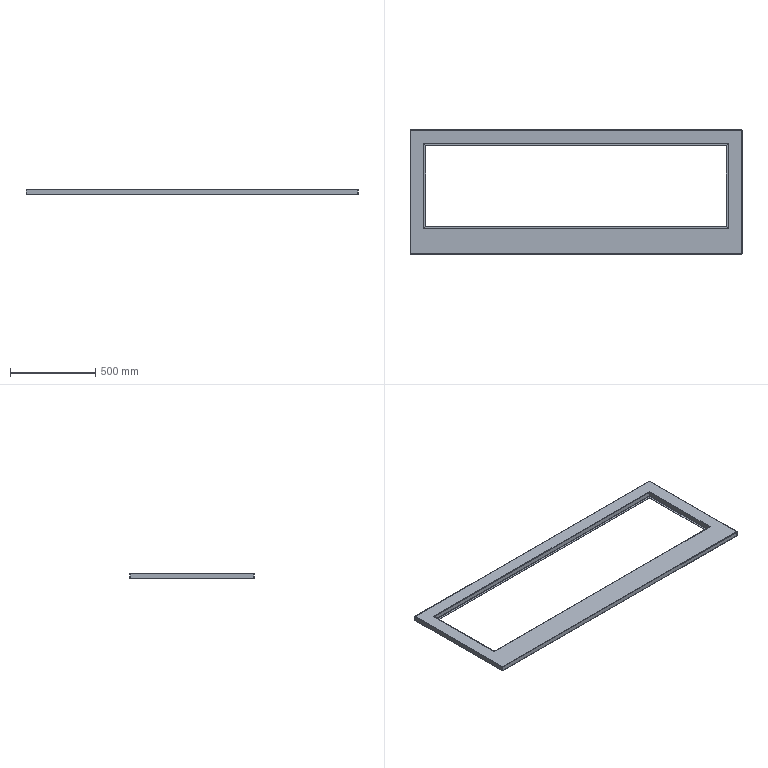Part | SolidWorks | features EdgeFlange 4, FlatPattern 1, HoleWzd 1, ICE 1, SMBaseFlange 1, SheetMetal 1 | 1 solid | 146 faces | box 1950 x 730 x 30 mm | volume 1438298 mm3 | plane 74 | cylinder 40 | spline 32 | commonest cylinder face diameters 1 x16 4 x16 5 x8